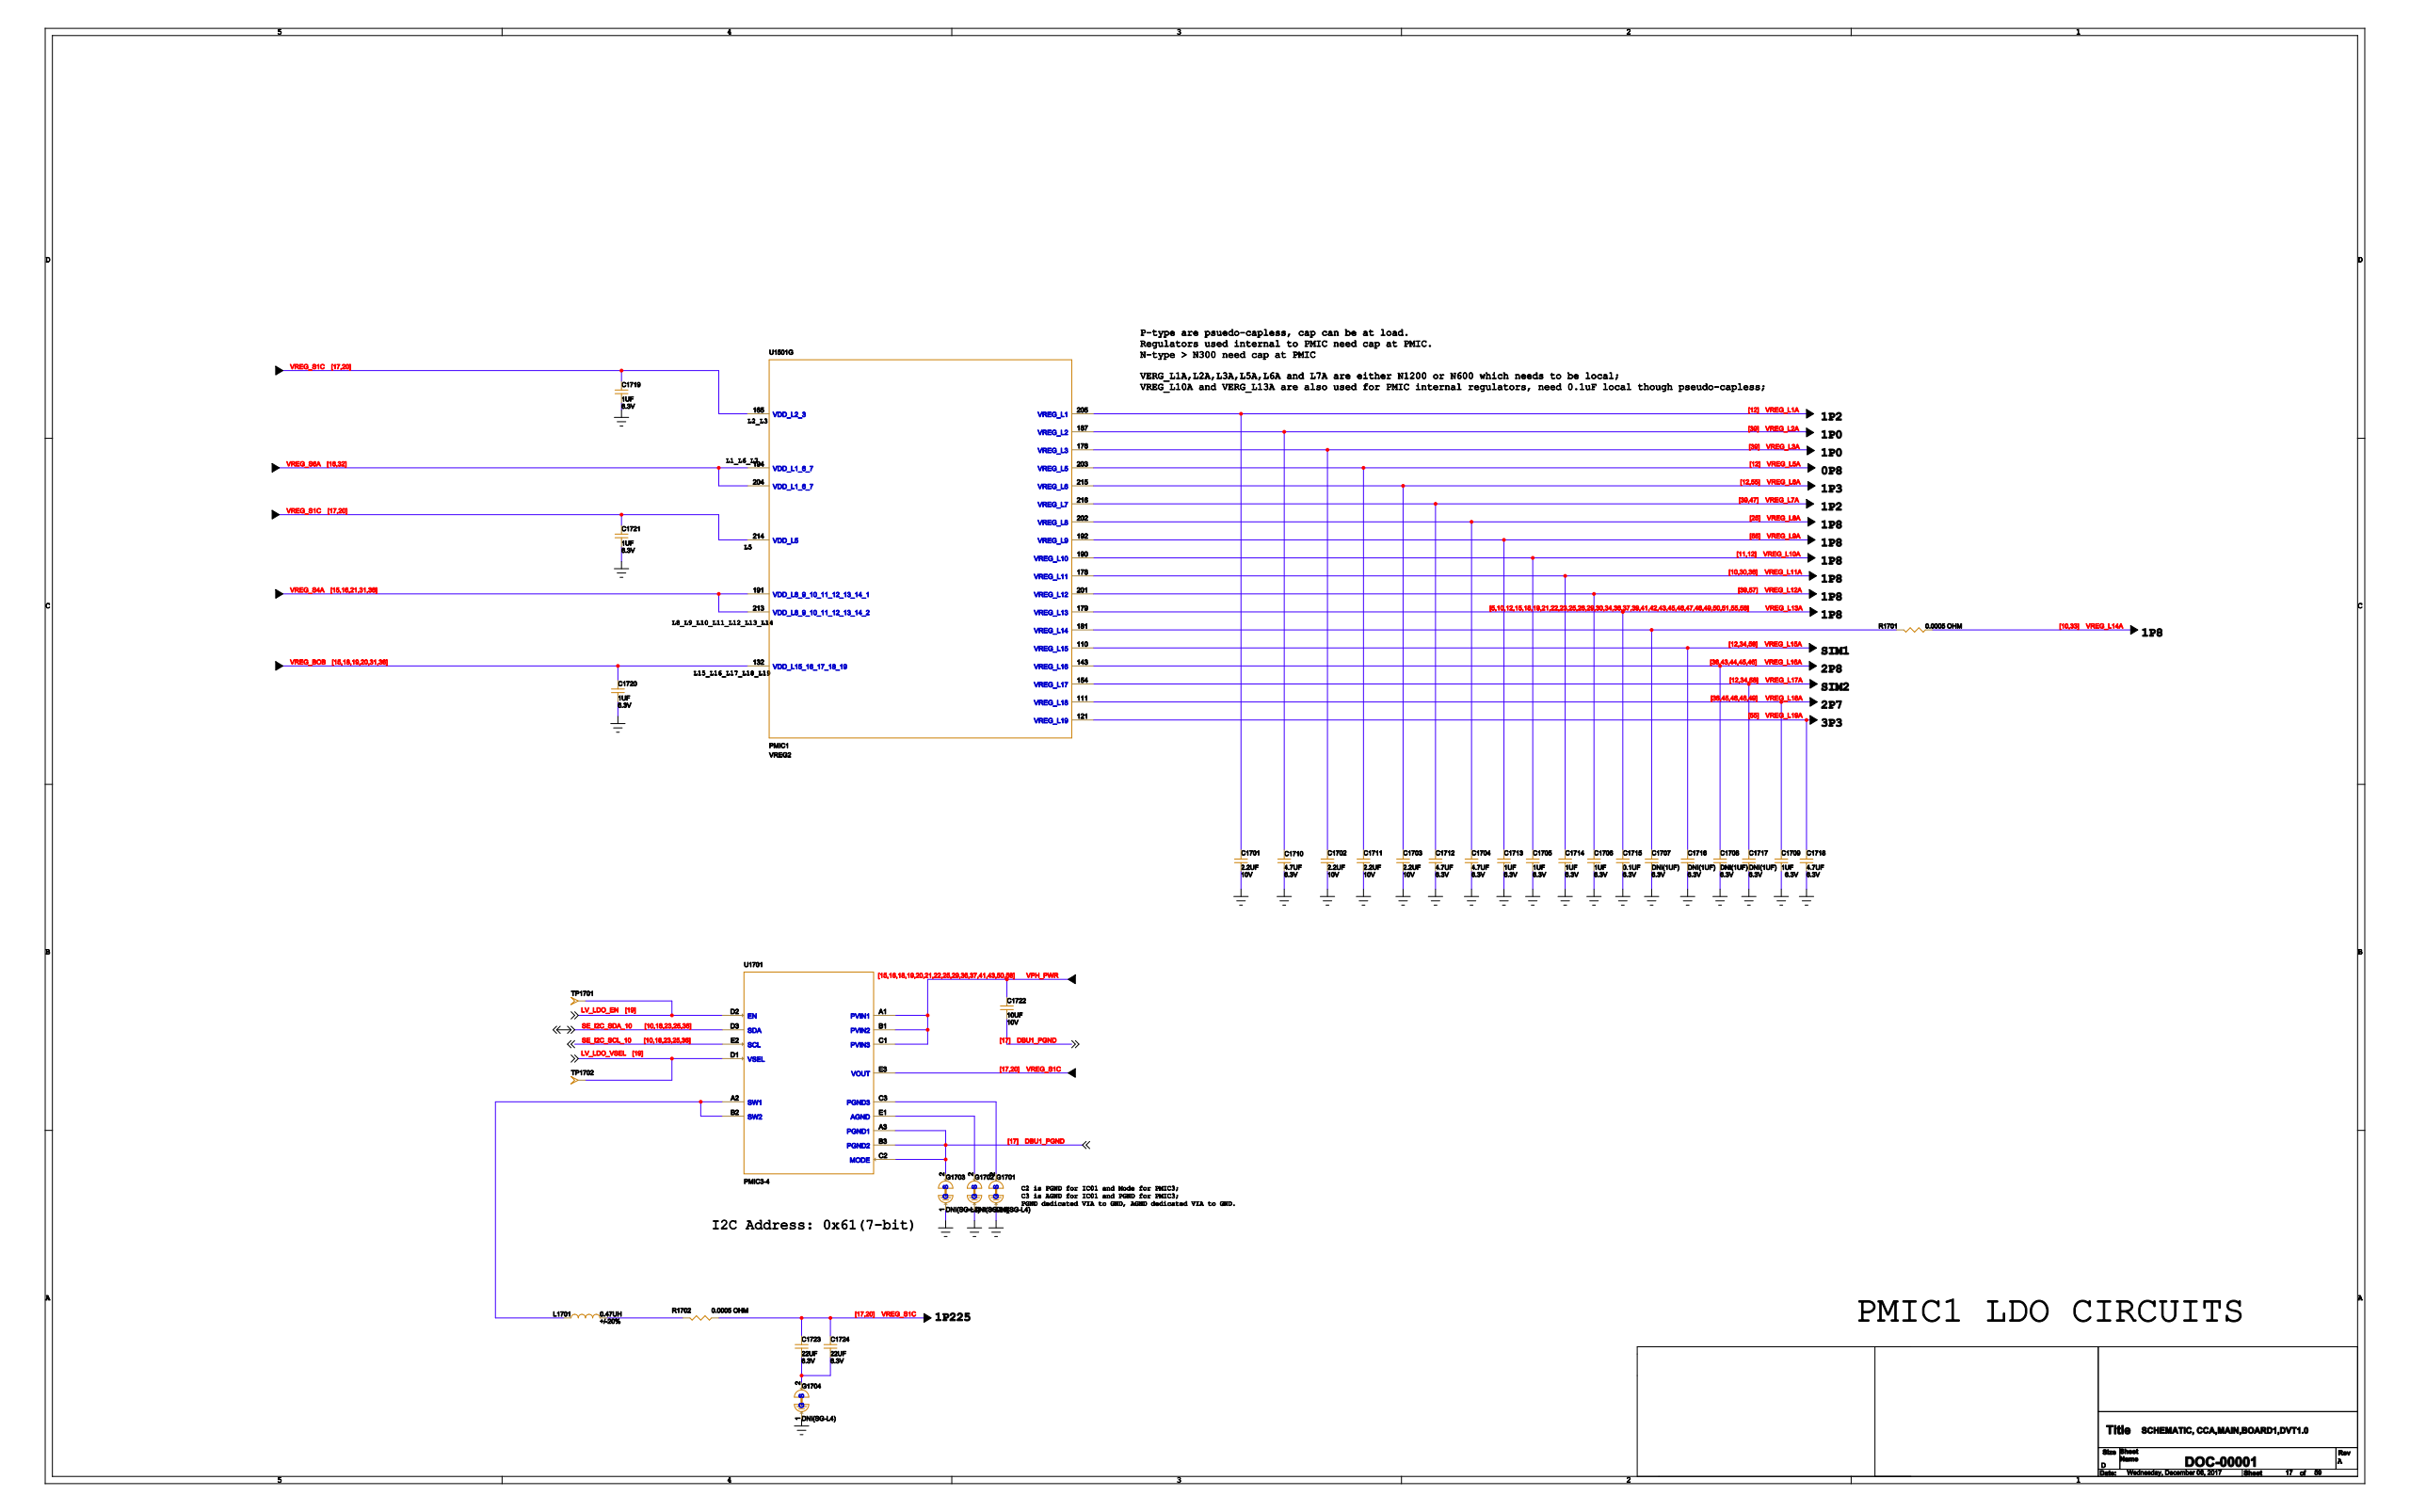Circuit board | KiCad | 1657 parts | 1365 nets | one sheet of the schematic
Parts on this sheet (reference | value | footprint):
C1701
C1702
C1703
C1704
C1705
C1706
C1707
C1708
C1709
C1710
C1711
C1712
C1713
C1714
C1715
C1716
C1717
C1718
C1719
C1720
C1721
C1722
C1723
C1724
G1701
G1702
G1703
G1704
L1701
R1701
R1702
TP1701
TP1702
U1501
U1701
Nets of these parts (net: part-pin ...):
GND: C1701-1 C1702-1 C1703-1 C1704-1 C1705-1 C1706-1 C1707-1 C1708-1 C1709-1 C1710-1 C1711-1 C1712-1 C1713-1 C1714-1 C1715-1 C1716-1 C1717-1 C1718-1 C1719-2 C1720-2 C1721-2 G1701-1 G1702-1 G1703-1 G1704-1
VREG_L13A: C1715-2 U1501-179
VPH_PWR: C1722-1 U1701-A1 U1701-B1 U1701-C1 U1501-3 U1501-15 U1501-20 U1501-25 U1501-37 U1501-42 U1501-47 U1501-55
VREG_L14A: R1701-2
VREG_BOB: C1720-1 U1501-132
SE_I2C_SCL_10: U1701-E2
SE_I2C_SDA_10: U1701-D3
VREG_L9A: C1713-2 U1501-192
DBU1_PGND: C1722-2 G1703-2 U1701-A3 U1701-B3 U1701-C2
VREG_L19A: C1718-2 U1501-121
VREG_L11A: C1714-2 U1501-178
VREG_S6A: U1501-194 U1501-204
VREG_L17A: C1717-2 U1501-154
VREG_L16A: C1708-2 U1501-143
VREG_L18A: C1709-2 U1501-111
VREG_L8A: C1704-2 U1501-202
VREG_S4A: U1501-191 U1501-213
VREG_L15A: C1716-2 U1501-110
VREG_S1C: C1719-1 C1721-1 C1723-1 C1724-1 R1702-2 U1701-E3 U1501-165 U1501-214
N20856628: C1723-2 C1724-2 G1704-2
VREG_L1A: C1701-2 U1501-205
VREG_L10A: C1705-2 U1501-190
VREG_L6A: C1703-2 U1501-215
VREG_L5A: C1711-2 U1501-203
N20856597: L1701-1 U1701-A2 U1701-B2
N20856632: L1701-2 R1702-1
N20856456: G1702-2 U1701-E1
N20856464: G1701-2 U1701-C3
LV_LDO_VSEL: TP1702-1 U1701-D1
LV_LDO_EN: TP1701-1 U1701-D2
VREG_L12A: C1706-2 U1501-201
VREG_L7A: C1712-2 U1501-216
VREG_L2A: C1710-2 U1501-187
N17092300: C1707-2 R1701-1 U1501-181
VREG_L3A: C1702-2 U1501-176